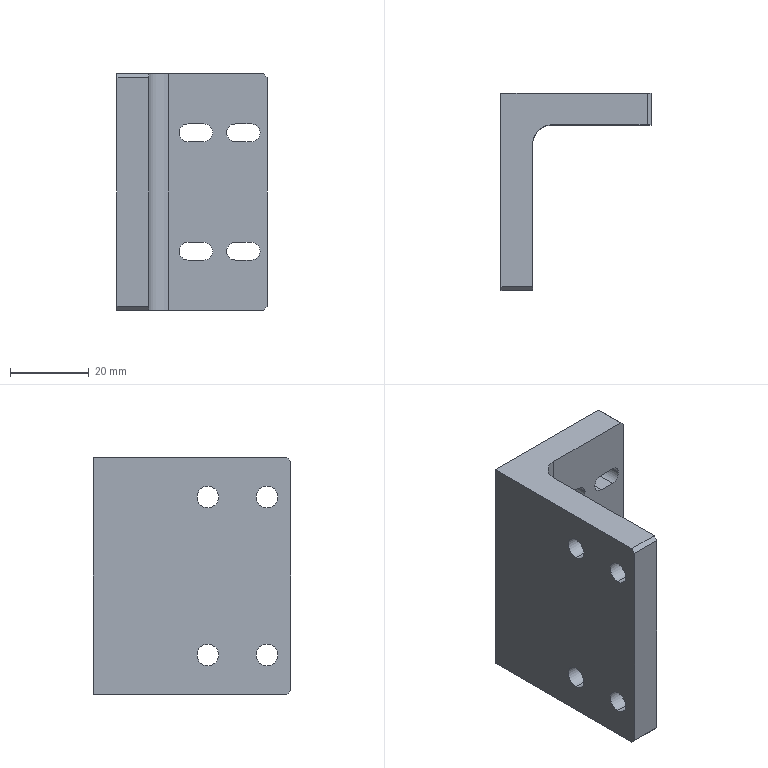Part | NX | features BREP 1 | 1 solid | 41 faces | box 38 x 50 x 60 mm | volume 36861 mm3 | cylinder 21 | plane 20 | commonest cylinder face diameters 4.5 x12 5.5 x8 10 x1
STEP:
#1=CARTESIAN_POINT('',(22.,50.,-12.75));
#2=VERTEX_POINT('',#1);
#3=CARTESIAN_POINT('',(24.25,50.,-15.));
#4=VERTEX_POINT('',#3);
#5=CARTESIAN_POINT('',(22.,50.,-15.));
#6=DIRECTION('',(0.,1.,0.));
#7=DIRECTION('',(0.,0.,1.));
#8=AXIS2_PLACEMENT_3D('',#5,#6,#7);
#9=CIRCLE('',#8,2.25);
#10=EDGE_CURVE('',#2,#4,#9,.T.);
#11=ORIENTED_EDGE('',*,*,#10,.T.);
#12=CARTESIAN_POINT('',(24.25,42.,-15.));
#13=VERTEX_POINT('',#12);
#14=CARTESIAN_POINT('',(24.25,59.,-15.));
#15=DIRECTION('',(0.,-1.,0.));
#16=VECTOR('',#15,1000.);
#17=LINE('',#14,#16);
#18=EDGE_CURVE('',#4,#13,#17,.T.);
#19=ORIENTED_EDGE('',*,*,#18,.T.);
#20=CARTESIAN_POINT('',(22.,42.,-12.75));
#21=VERTEX_POINT('',#20);
#22=CARTESIAN_POINT('',(22.,42.,-15.));
#23=DIRECTION('',(0.,-1.,0.));
#24=DIRECTION('',(1.,0.,0.));
#25=AXIS2_PLACEMENT_3D('',#22,#23,#24);
#26=CIRCLE('',#25,2.25);
#27=EDGE_CURVE('',#13,#21,#26,.T.);
#28=ORIENTED_EDGE('',*,*,#27,.T.);
#29=CARTESIAN_POINT('',(22.,59.,-12.75));
#30=DIRECTION('',(0.,-1.,0.));
#31=VECTOR('',#30,1000.);
#32=LINE('',#29,#31);
#33=EDGE_CURVE('',#2,#21,#32,.T.);
#34=ORIENTED_EDGE('',*,*,#33,.F.);
#35=EDGE_LOOP('',(#11,#19,#28,#34));
#36=FACE_BOUND('',#35,.T.);
#37=CARTESIAN_POINT('',(22.,59.,-15.));
#38=DIRECTION('',(0.,-1.,0.));
#39=DIRECTION('',(1.,0.,0.));
#40=AXIS2_PLACEMENT_3D('',#37,#38,#39);
#41=CYLINDRICAL_SURFACE('',#40,2.25);
#42=ADVANCED_FACE('',(#36),#41,.F.);
#43=CARTESIAN_POINT('',(34.,50.,-12.75));
#44=VERTEX_POINT('',#43);
#45=CARTESIAN_POINT('',(36.25,50.,-15.));
#46=VERTEX_POINT('',#45);
#47=CARTESIAN_POINT('',(34.,50.,-15.));
#48=DIRECTION('',(0.,1.,0.));
#49=DIRECTION('',(0.,0.,1.));
#50=AXIS2_PLACEMENT_3D('',#47,#48,#49);
#51=CIRCLE('',#50,2.25);
#52=EDGE_CURVE('',#44,#46,#51,.T.);
#53=ORIENTED_EDGE('',*,*,#52,.T.);
#54=CARTESIAN_POINT('',(36.25,42.,-15.));
#55=VERTEX_POINT('',#54);
#56=CARTESIAN_POINT('',(36.25,59.,-15.));
#57=DIRECTION('',(0.,-1.,0.));
#58=VECTOR('',#57,1000.);
#59=LINE('',#56,#58);
#60=EDGE_CURVE('',#46,#55,#59,.T.);
#61=ORIENTED_EDGE('',*,*,#60,.T.);
#62=CARTESIAN_POINT('',(34.,42.,-12.75));
#63=VERTEX_POINT('',#62);
#64=CARTESIAN_POINT('',(34.,42.,-15.));
#65=DIRECTION('',(0.,-1.,0.));
#66=DIRECTION('',(1.,0.,0.));
#67=AXIS2_PLACEMENT_3D('',#64,#65,#66);
#68=CIRCLE('',#67,2.25);
#69=EDGE_CURVE('',#55,#63,#68,.T.);
#70=ORIENTED_EDGE('',*,*,#69,.T.);
#71=CARTESIAN_POINT('',(34.,59.,-12.75));
#72=DIRECTION('',(0.,-1.,0.));
#73=VECTOR('',#72,1000.);
#74=LINE('',#71,#73);
#75=EDGE_CURVE('',#44,#63,#74,.T.);
#76=ORIENTED_EDGE('',*,*,#75,.F.);
#77=EDGE_LOOP('',(#53,#61,#70,#76));
#78=FACE_BOUND('',#77,.T.);
#79=CARTESIAN_POINT('',(34.,59.,-15.));
#80=DIRECTION('',(0.,-1.,0.));
#81=DIRECTION('',(1.,0.,0.));
#82=AXIS2_PLACEMENT_3D('',#79,#80,#81);
#83=CYLINDRICAL_SURFACE('',#82,2.25);
#84=ADVANCED_FACE('',(#78),#83,.F.);
#85=CARTESIAN_POINT('',(22.,50.,17.25));
#86=VERTEX_POINT('',#85);
#87=CARTESIAN_POINT('',(24.25,50.,15.));
#88=VERTEX_POINT('',#87);
#89=CARTESIAN_POINT('',(22.,50.,15.));
#90=DIRECTION('',(0.,1.,0.));
#91=DIRECTION('',(0.,0.,1.));
#92=AXIS2_PLACEMENT_3D('',#89,#90,#91);
#93=CIRCLE('',#92,2.25);
#94=EDGE_CURVE('',#86,#88,#93,.T.);
#95=ORIENTED_EDGE('',*,*,#94,.T.);
#96=CARTESIAN_POINT('',(24.25,42.,15.));
#97=VERTEX_POINT('',#96);
#98=CARTESIAN_POINT('',(24.25,59.,15.));
#99=DIRECTION('',(0.,-1.,0.));
#100=VECTOR('',#99,1000.);
#101=LINE('',#98,#100);
#102=EDGE_CURVE('',#88,#97,#101,.T.);
#103=ORIENTED_EDGE('',*,*,#102,.T.);
#104=CARTESIAN_POINT('',(22.,42.,17.25));
#105=VERTEX_POINT('',#104);
#106=CARTESIAN_POINT('',(22.,42.,15.));
#107=DIRECTION('',(0.,-1.,0.));
#108=DIRECTION('',(1.,0.,0.));
#109=AXIS2_PLACEMENT_3D('',#106,#107,#108);
#110=CIRCLE('',#109,2.25);
#111=EDGE_CURVE('',#97,#105,#110,.T.);
#112=ORIENTED_EDGE('',*,*,#111,.T.);
#113=CARTESIAN_POINT('',(22.,59.,17.25));
#114=DIRECTION('',(0.,-1.,0.));
#115=VECTOR('',#114,1000.);
#116=LINE('',#113,#115);
#117=EDGE_CURVE('',#86,#105,#116,.T.);
#118=ORIENTED_EDGE('',*,*,#117,.F.);
#119=EDGE_LOOP('',(#95,#103,#112,#118));
#120=FACE_BOUND('',#119,.T.);
#121=CARTESIAN_POINT('',(22.,59.,15.));
#122=DIRECTION('',(0.,-1.,0.));
#123=DIRECTION('',(1.,0.,0.));
#124=AXIS2_PLACEMENT_3D('',#121,#122,#123);
#125=CYLINDRICAL_SURFACE('',#124,2.25);
#126=ADVANCED_FACE('',(#120),#125,.F.);
#127=CARTESIAN_POINT('',(34.,50.,17.25));
#128=VERTEX_POINT('',#127);
#129=CARTESIAN_POINT('',(36.25,50.,15.));
#130=VERTEX_POINT('',#129);
#131=CARTESIAN_POINT('',(34.,50.,15.));
#132=DIRECTION('',(0.,1.,0.));
#133=DIRECTION('',(0.,0.,1.));
#134=AXIS2_PLACEMENT_3D('',#131,#132,#133);
#135=CIRCLE('',#134,2.25);
#136=EDGE_CURVE('',#128,#130,#135,.T.);
#137=ORIENTED_EDGE('',*,*,#136,.T.);
#138=CARTESIAN_POINT('',(36.25,42.,15.));
#139=VERTEX_POINT('',#138);
#140=CARTESIAN_POINT('',(36.25,59.,15.));
#141=DIRECTION('',(0.,-1.,0.));
#142=VECTOR('',#141,1000.);
#143=LINE('',#140,#142);
#144=EDGE_CURVE('',#130,#139,#143,.T.);
#145=ORIENTED_EDGE('',*,*,#144,.T.);
#146=CARTESIAN_POINT('',(34.,42.,17.25));
#147=VERTEX_POINT('',#146);
#148=CARTESIAN_POINT('',(34.,42.,15.));
#149=DIRECTION('',(0.,-1.,0.));
#150=DIRECTION('',(1.,0.,0.));
#151=AXIS2_PLACEMENT_3D('',#148,#149,#150);
#152=CIRCLE('',#151,2.25);
#153=EDGE_CURVE('',#139,#147,#152,.T.);
#154=ORIENTED_EDGE('',*,*,#153,.T.);
#155=CARTESIAN_POINT('',(34.,59.,17.25));
#156=DIRECTION('',(0.,-1.,0.));
#157=VECTOR('',#156,1000.);
#158=LINE('',#155,#157);
#159=EDGE_CURVE('',#128,#147,#158,.T.);
#160=ORIENTED_EDGE('',*,*,#159,.F.);
#161=EDGE_LOOP('',(#137,#145,#154,#160));
#162=FACE_BOUND('',#161,.T.);
#163=CARTESIAN_POINT('',(34.,59.,15.));
#164=DIRECTION('',(0.,-1.,0.));
#165=DIRECTION('',(1.,0.,0.));
#166=AXIS2_PLACEMENT_3D('',#163,#164,#165);
#167=CYLINDRICAL_SURFACE('',#166,2.25);
#168=ADVANCED_FACE('',(#162),#167,.F.);
#169=CARTESIAN_POINT('',(0.,21.,17.25));
#170=VERTEX_POINT('',#169);
#171=CARTESIAN_POINT('',(0.,21.,22.75));
#172=VERTEX_POINT('',#171);
#173=CARTESIAN_POINT('',(0.,21.,20.));
#174=DIRECTION('',(-1.,0.,0.));
#175=DIRECTION('',(0.,0.,1.));
#176=AXIS2_PLACEMENT_3D('',#173,#174,#175);
#177=CIRCLE('',#176,2.75);
#178=EDGE_CURVE('',#170,#172,#177,.T.);
#179=ORIENTED_EDGE('',*,*,#178,.T.);
#180=CARTESIAN_POINT('',(8.,21.,22.75));
#181=VERTEX_POINT('',#180);
#182=CARTESIAN_POINT('',(8.,21.,22.75));
#183=DIRECTION('',(1.,0.,0.));
#184=VECTOR('',#183,1000.);
#185=LINE('',#182,#184);
#186=EDGE_CURVE('',#172,#181,#185,.T.);
#187=ORIENTED_EDGE('',*,*,#186,.T.);
#188=CARTESIAN_POINT('',(8.,21.,17.25));
#189=VERTEX_POINT('',#188);
#190=CARTESIAN_POINT('',(8.,21.,20.));
#191=DIRECTION('',(1.,0.,0.));
#192=DIRECTION('',(0.,0.,-1.));
#193=AXIS2_PLACEMENT_3D('',#190,#191,#192);
#194=CIRCLE('',#193,2.75);
#195=EDGE_CURVE('',#181,#189,#194,.T.);
#196=ORIENTED_EDGE('',*,*,#195,.T.);
#197=CARTESIAN_POINT('',(8.,21.,17.25));
#198=DIRECTION('',(1.,0.,0.));
#199=VECTOR('',#198,1000.);
#200=LINE('',#197,#199);
#201=EDGE_CURVE('',#170,#189,#200,.T.);
#202=ORIENTED_EDGE('',*,*,#201,.F.);
#203=EDGE_LOOP('',(#179,#187,#196,#202));
#204=FACE_BOUND('',#203,.T.);
#205=CARTESIAN_POINT('',(8.,21.,20.));
#206=DIRECTION('',(1.,0.,0.));
#207=DIRECTION('',(0.,0.,-1.));
#208=AXIS2_PLACEMENT_3D('',#205,#206,#207);
#209=CYLINDRICAL_SURFACE('',#208,2.75);
#210=ADVANCED_FACE('',(#204),#209,.F.);
#211=CARTESIAN_POINT('',(0.,6.,17.25));
#212=VERTEX_POINT('',#211);
#213=CARTESIAN_POINT('',(0.,6.,22.75));
#214=VERTEX_POINT('',#213);
#215=CARTESIAN_POINT('',(0.,6.,20.));
#216=DIRECTION('',(-1.,0.,0.));
#217=DIRECTION('',(0.,0.,1.));
#218=AXIS2_PLACEMENT_3D('',#215,#216,#217);
#219=CIRCLE('',#218,2.75);
#220=EDGE_CURVE('',#212,#214,#219,.T.);
#221=ORIENTED_EDGE('',*,*,#220,.T.);
#222=CARTESIAN_POINT('',(8.,6.,22.75));
#223=VERTEX_POINT('',#222);
#224=CARTESIAN_POINT('',(8.,6.,22.75));
#225=DIRECTION('',(1.,0.,0.));
#226=VECTOR('',#225,1000.);
#227=LINE('',#224,#226);
#228=EDGE_CURVE('',#214,#223,#227,.T.);
#229=ORIENTED_EDGE('',*,*,#228,.T.);
#230=CARTESIAN_POINT('',(8.,6.,17.25));
#231=VERTEX_POINT('',#230);
#232=CARTESIAN_POINT('',(8.,6.,20.));
#233=DIRECTION('',(1.,0.,0.));
#234=DIRECTION('',(0.,0.,-1.));
#235=AXIS2_PLACEMENT_3D('',#232,#233,#234);
#236=CIRCLE('',#235,2.75);
#237=EDGE_CURVE('',#223,#231,#236,.T.);
#238=ORIENTED_EDGE('',*,*,#237,.T.);
#239=CARTESIAN_POINT('',(8.,6.,17.25));
#240=DIRECTION('',(1.,0.,0.));
#241=VECTOR('',#240,1000.);
#242=LINE('',#239,#241);
#243=EDGE_CURVE('',#212,#231,#242,.T.);
#244=ORIENTED_EDGE('',*,*,#243,.F.);
#245=EDGE_LOOP('',(#221,#229,#238,#244));
#246=FACE_BOUND('',#245,.T.);
#247=CARTESIAN_POINT('',(8.,6.,20.));
#248=DIRECTION('',(1.,0.,0.));
#249=DIRECTION('',(0.,0.,-1.));
#250=AXIS2_PLACEMENT_3D('',#247,#248,#249);
#251=CYLINDRICAL_SURFACE('',#250,2.75);
#252=ADVANCED_FACE('',(#246),#251,.F.);
#253=CARTESIAN_POINT('',(0.,6.,-22.75));
#254=VERTEX_POINT('',#253);
#255=CARTESIAN_POINT('',(0.,6.,-17.25));
#256=VERTEX_POINT('',#255);
#257=CARTESIAN_POINT('',(0.,6.,-20.));
#258=DIRECTION('',(-1.,0.,0.));
#259=DIRECTION('',(0.,0.,1.));
#260=AXIS2_PLACEMENT_3D('',#257,#258,#259);
#261=CIRCLE('',#260,2.75);
#262=EDGE_CURVE('',#254,#256,#261,.T.);
#263=ORIENTED_EDGE('',*,*,#262,.T.);
#264=CARTESIAN_POINT('',(8.,6.,-17.25));
#265=VERTEX_POINT('',#264);
#266=CARTESIAN_POINT('',(8.,6.,-17.25));
#267=DIRECTION('',(1.,0.,0.));
#268=VECTOR('',#267,1000.);
#269=LINE('',#266,#268);
#270=EDGE_CURVE('',#256,#265,#269,.T.);
#271=ORIENTED_EDGE('',*,*,#270,.T.);
#272=CARTESIAN_POINT('',(8.,6.,-22.75));
#273=VERTEX_POINT('',#272);
#274=CARTESIAN_POINT('',(8.,6.,-20.));
#275=DIRECTION('',(1.,0.,0.));
#276=DIRECTION('',(0.,0.,-1.));
#277=AXIS2_PLACEMENT_3D('',#274,#275,#276);
#278=CIRCLE('',#277,2.75);
#279=EDGE_CURVE('',#265,#273,#278,.T.);
#280=ORIENTED_EDGE('',*,*,#279,.T.);
#281=CARTESIAN_POINT('',(8.,6.,-22.75));
#282=DIRECTION('',(1.,0.,0.));
#283=VECTOR('',#282,1000.);
#284=LINE('',#281,#283);
#285=EDGE_CURVE('',#254,#273,#284,.T.);
#286=ORIENTED_EDGE('',*,*,#285,.F.);
#287=EDGE_LOOP('',(#263,#271,#280,#286));
#288=FACE_BOUND('',#287,.T.);
#289=CARTESIAN_POINT('',(8.,6.,-20.));
#290=DIRECTION('',(1.,0.,0.));
#291=DIRECTION('',(0.,0.,-1.));
#292=AXIS2_PLACEMENT_3D('',#289,#290,#291);
#293=CYLINDRICAL_SURFACE('',#292,2.75);
#294=ADVANCED_FACE('',(#288),#293,.F.);
#295=CARTESIAN_POINT('',(0.,21.,-22.75));
#296=VERTEX_POINT('',#295);
#297=CARTESIAN_POINT('',(0.,21.,-17.25));
#298=VERTEX_POINT('',#297);
#299=CARTESIAN_POINT('',(0.,21.,-20.));
#300=DIRECTION('',(-1.,0.,0.));
#301=DIRECTION('',(0.,0.,1.));
#302=AXIS2_PLACEMENT_3D('',#299,#300,#301);
#303=CIRCLE('',#302,2.75);
#304=EDGE_CURVE('',#296,#298,#303,.T.);
#305=ORIENTED_EDGE('',*,*,#304,.T.);
#306=CARTESIAN_POINT('',(8.,21.,-17.25));
#307=VERTEX_POINT('',#306);
#308=CARTESIAN_POINT('',(8.,21.,-17.25));
#309=DIRECTION('',(1.,0.,0.));
#310=VECTOR('',#309,1000.);
#311=LINE('',#308,#310);
#312=EDGE_CURVE('',#298,#307,#311,.T.);
#313=ORIENTED_EDGE('',*,*,#312,.T.);
#314=CARTESIAN_POINT('',(8.,21.,-22.75));
#315=VERTEX_POINT('',#314);
#316=CARTESIAN_POINT('',(8.,21.,-20.));
#317=DIRECTION('',(1.,0.,0.));
#318=DIRECTION('',(0.,0.,-1.));
#319=AXIS2_PLACEMENT_3D('',#316,#317,#318);
#320=CIRCLE('',#319,2.75);
#321=EDGE_CURVE('',#307,#315,#320,.T.);
#322=ORIENTED_EDGE('',*,*,#321,.T.);
#323=CARTESIAN_POINT('',(8.,21.,-22.75));
#324=DIRECTION('',(1.,0.,0.));
#325=VECTOR('',#324,1000.);
#326=LINE('',#323,#325);
#327=EDGE_CURVE('',#296,#315,#326,.T.);
#328=ORIENTED_EDGE('',*,*,#327,.F.);
#329=EDGE_LOOP('',(#305,#313,#322,#328));
#330=FACE_BOUND('',#329,.T.);
#331=CARTESIAN_POINT('',(8.,21.,-20.));
#332=DIRECTION('',(1.,0.,0.));
#333=DIRECTION('',(0.,0.,-1.));
#334=AXIS2_PLACEMENT_3D('',#331,#332,#333);
#335=CYLINDRICAL_SURFACE('',#334,2.75);
#336=ADVANCED_FACE('',(#330),#335,.F.);
#337=CARTESIAN_POINT('',(8.,0.,29.));
#338=VERTEX_POINT('',#337);
#339=CARTESIAN_POINT('',(8.,0.,-29.));
#340=VERTEX_POINT('',#339);
#341=CARTESIAN_POINT('',(8.,0.,30.));
#342=DIRECTION('',(0.,0.,-1.));
#343=VECTOR('',#342,1000.);
#344=LINE('',#341,#343);
#345=EDGE_CURVE('',#338,#340,#344,.T.);
#346=ORIENTED_EDGE('',*,*,#345,.T.);
#347=CARTESIAN_POINT('',(8.,1.,-30.));
#348=VERTEX_POINT('',#347);
#349=CARTESIAN_POINT('',(8.,-29.5,0.5));
#350=DIRECTION('',(0.,0.7071,-0.7071));
#351=VECTOR('',#350,1000.);
#352=LINE('',#349,#351);
#353=EDGE_CURVE('',#340,#348,#352,.T.);
#354=ORIENTED_EDGE('',*,*,#353,.T.);
#355=CARTESIAN_POINT('',(8.,37.,-30.));
#356=VERTEX_POINT('',#355);
#357=CARTESIAN_POINT('',(8.,0.,-30.));
#358=DIRECTION('',(0.,-1.,0.));
#359=VECTOR('',#358,1000.);
#360=LINE('',#357,#359);
#361=EDGE_CURVE('',#356,#348,#360,.T.);
#362=ORIENTED_EDGE('',*,*,#361,.F.);
#363=CARTESIAN_POINT('',(8.,37.,30.));
#364=VERTEX_POINT('',#363);
#365=CARTESIAN_POINT('',(8.,37.,30.));
#366=DIRECTION('',(0.,0.,-1.));
#367=VECTOR('',#366,1000.);
#368=LINE('',#365,#367);
#369=EDGE_CURVE('',#364,#356,#368,.T.);
#370=ORIENTED_EDGE('',*,*,#369,.F.);
#371=CARTESIAN_POINT('',(8.,1.,30.));
#372=VERTEX_POINT('',#371);
#373=CARTESIAN_POINT('',(8.,0.,30.));
#374=DIRECTION('',(0.,-1.,0.));
#375=VECTOR('',#374,1000.);
#376=LINE('',#373,#375);
#377=EDGE_CURVE('',#364,#372,#376,.T.);
#378=ORIENTED_EDGE('',*,*,#377,.T.);
#379=CARTESIAN_POINT('',(8.,0.5,29.5));
#380=DIRECTION('',(0.,-0.7071,-0.7071));
#381=VECTOR('',#380,1000.);
#382=LINE('',#379,#381);
#383=EDGE_CURVE('',#372,#338,#382,.T.);
#384=ORIENTED_EDGE('',*,*,#383,.T.);
#385=EDGE_LOOP('',(#346,#354,#362,#370,#378,#384));
#386=FACE_BOUND('',#385,.T.);
#387=CARTESIAN_POINT('',(8.,21.,20.));
#388=DIRECTION('',(1.,0.,0.));
#389=DIRECTION('',(0.,0.,-1.));
#390=AXIS2_PLACEMENT_3D('',#387,#388,#389);
#391=CIRCLE('',#390,2.75);
#392=EDGE_CURVE('',#189,#181,#391,.T.);
#393=ORIENTED_EDGE('',*,*,#392,.F.);
#394=ORIENTED_EDGE('',*,*,#195,.F.);
#395=EDGE_LOOP('',(#393,#394));
#396=FACE_BOUND('',#395,.T.);
#397=CARTESIAN_POINT('',(8.,6.,20.));
#398=DIRECTION('',(1.,0.,0.));
#399=DIRECTION('',(0.,0.,-1.));
#400=AXIS2_PLACEMENT_3D('',#397,#398,#399);
#401=CIRCLE('',#400,2.75);
#402=EDGE_CURVE('',#231,#223,#401,.T.);
#403=ORIENTED_EDGE('',*,*,#402,.F.);
#404=ORIENTED_EDGE('',*,*,#237,.F.);
#405=EDGE_LOOP('',(#403,#404));
#406=FACE_BOUND('',#405,.T.);
#407=CARTESIAN_POINT('',(8.,6.,-20.));
#408=DIRECTION('',(1.,0.,0.));
#409=DIRECTION('',(0.,0.,-1.));
#410=AXIS2_PLACEMENT_3D('',#407,#408,#409);
#411=CIRCLE('',#410,2.75);
#412=EDGE_CURVE('',#273,#265,#411,.T.);
#413=ORIENTED_EDGE('',*,*,#412,.F.);
#414=ORIENTED_EDGE('',*,*,#279,.F.);
#415=EDGE_LOOP('',(#413,#414));
#416=FACE_BOUND('',#415,.T.);
#417=CARTESIAN_POINT('',(8.,21.,-20.));
#418=DIRECTION('',(1.,0.,0.));
#419=DIRECTION('',(0.,0.,-1.));
#420=AXIS2_PLACEMENT_3D('',#417,#418,#419);
#421=CIRCLE('',#420,2.75);
#422=EDGE_CURVE('',#315,#307,#421,.T.);
#423=ORIENTED_EDGE('',*,*,#422,.F.);
#424=ORIENTED_EDGE('',*,*,#321,.F.);
#425=EDGE_LOOP('',(#423,#424));
#426=FACE_BOUND('',#425,.T.);
#427=CARTESIAN_POINT('',(8.,0.,30.));
#428=DIRECTION('',(1.,0.,0.));
#429=DIRECTION('',(0.,1.,0.));
#430=AXIS2_PLACEMENT_3D('',#427,#428,#429);
#431=PLANE('',#430);
#432=ADVANCED_FACE('',(#386,#396,#406,#416,#426),#431,.T.);
#433=CARTESIAN_POINT('',(13.,42.,-30.));
#434=VERTEX_POINT('',#433);
#435=CARTESIAN_POINT('',(13.,37.,-30.));
#436=DIRECTION('',(0.,0.,-1.));
#437=DIRECTION('',(1.,0.,0.));
#438=AXIS2_PLACEMENT_3D('',#435,#436,#437);
#439=CIRCLE('',#438,5.);
#440=EDGE_CURVE('',#356,#434,#439,.T.);
#441=ORIENTED_EDGE('',*,*,#440,.T.);
#442=CARTESIAN_POINT('',(13.,42.,30.));
#443=VERTEX_POINT('',#442);
#444=CARTESIAN_POINT('',(13.,42.,30.));
#445=DIRECTION('',(0.,0.,-1.));
#446=VECTOR('',#445,1000.);
#447=LINE('',#444,#446);
#448=EDGE_CURVE('',#443,#434,#447,.T.);
#449=ORIENTED_EDGE('',*,*,#448,.F.);
#450=CARTESIAN_POINT('',(13.,37.,30.));
#451=DIRECTION('',(0.,0.,-1.));
#452=DIRECTION('',(1.,0.,0.));
#453=AXIS2_PLACEMENT_3D('',#450,#451,#452);
#454=CIRCLE('',#453,5.);
#455=EDGE_CURVE('',#364,#443,#454,.T.);
#456=ORIENTED_EDGE('',*,*,#455,.F.);
#457=ORIENTED_EDGE('',*,*,#369,.T.);
#458=EDGE_LOOP('',(#441,#449,#456,#457));
#459=FACE_BOUND('',#458,.T.);
#460=CARTESIAN_POINT('',(13.,37.,30.));
#461=DIRECTION('',(0.,0.,-1.));
#462=DIRECTION('',(-1.,0.,0.));
#463=AXIS2_PLACEMENT_3D('',#460,#461,#462);
#464=CYLINDRICAL_SURFACE('',#463,5.);
#465=ADVANCED_FACE('',(#459),#464,.F.);
#466=CARTESIAN_POINT('',(38.,42.,29.));
#467=VERTEX_POINT('',#466);
#468=CARTESIAN_POINT('',(38.,42.,-29.));
#469=VERTEX_POINT('',#468);
#470=CARTESIAN_POINT('',(38.,42.,30.));
#471=DIRECTION('',(0.,0.,-1.));
#472=VECTOR('',#471,1000.);
#473=LINE('',#470,#472);
#474=EDGE_CURVE('',#467,#469,#473,.T.);
#475=ORIENTED_EDGE('',*,*,#474,.F.);
#476=CARTESIAN_POINT('',(37.,42.,30.));
#477=VERTEX_POINT('',#476);
#478=CARTESIAN_POINT('',(18.5,42.,48.5));
#479=DIRECTION('',(-0.7071,0.,0.7071));
#480=VECTOR('',#479,1000.);
#481=LINE('',#478,#480);
#482=EDGE_CURVE('',#467,#477,#481,.T.);
#483=ORIENTED_EDGE('',*,*,#482,.T.);
#484=CARTESIAN_POINT('',(0.,42.,30.));
#485=DIRECTION('',(-1.,0.,0.));
#486=VECTOR('',#485,1000.);
#487=LINE('',#484,#486);
#488=EDGE_CURVE('',#477,#443,#487,.T.);
#489=ORIENTED_EDGE('',*,*,#488,.T.);
#490=ORIENTED_EDGE('',*,*,#448,.T.);
#491=CARTESIAN_POINT('',(37.,42.,-30.));
#492=VERTEX_POINT('',#491);
#493=CARTESIAN_POINT('',(0.,42.,-30.));
#494=DIRECTION('',(-1.,0.,0.));
#495=VECTOR('',#494,1000.);
#496=LINE('',#493,#495);
#497=EDGE_CURVE('',#492,#434,#496,.T.);
#498=ORIENTED_EDGE('',*,*,#497,.F.);
#499=CARTESIAN_POINT('',(48.5,42.,-18.5));
#500=DIRECTION('',(0.7071,0.,0.7071));
#501=VECTOR('',#500,1000.);
#502=LINE('',#499,#501);
#503=EDGE_CURVE('',#492,#469,#502,.T.);
#504=ORIENTED_EDGE('',*,*,#503,.T.);
#505=EDGE_LOOP('',(#475,#483,#489,#490,#498,#504));
#506=FACE_BOUND('',#505,.T.);
#507=CARTESIAN_POINT('',(18.,42.,-12.75));
#508=VERTEX_POINT('',#507);
#509=CARTESIAN_POINT('',(18.,42.,-12.75));
#510=DIRECTION('',(-1.,0.,0.));
#511=VECTOR('',#510,1000.);
#512=LINE('',#509,#511);
#513=EDGE_CURVE('',#21,#508,#512,.T.);
#514=ORIENTED_EDGE('',*,*,#513,.F.);
#515=ORIENTED_EDGE('',*,*,#27,.F.);
#516=CARTESIAN_POINT('',(22.,42.,-17.25));
#517=VERTEX_POINT('',#516);
#518=CARTESIAN_POINT('',(22.,42.,-15.));
#519=DIRECTION('',(0.,-1.,0.));
#520=DIRECTION('',(1.,0.,0.));
#521=AXIS2_PLACEMENT_3D('',#518,#519,#520);
#522=CIRCLE('',#521,2.25);
#523=EDGE_CURVE('',#517,#13,#522,.T.);
#524=ORIENTED_EDGE('',*,*,#523,.F.);
#525=CARTESIAN_POINT('',(18.,42.,-17.25));
#526=VERTEX_POINT('',#525);
#527=CARTESIAN_POINT('',(18.,42.,-17.25));
#528=DIRECTION('',(1.,0.,0.));
#529=VECTOR('',#528,1000.);
#530=LINE('',#527,#529);
#531=EDGE_CURVE('',#526,#517,#530,.T.);
#532=ORIENTED_EDGE('',*,*,#531,.F.);
#533=CARTESIAN_POINT('',(18.,42.,-15.));
#534=DIRECTION('',(0.,-1.,0.));
#535=DIRECTION('',(1.,0.,0.));
#536=AXIS2_PLACEMENT_3D('',#533,#534,#535);
#537=CIRCLE('',#536,2.25);
#538=EDGE_CURVE('',#508,#526,#537,.T.);
#539=ORIENTED_EDGE('',*,*,#538,.F.);
#540=EDGE_LOOP('',(#514,#515,#524,#532,#539));
#541=FACE_BOUND('',#540,.T.);
#542=CARTESIAN_POINT('',(30.,42.,-12.75));
#543=VERTEX_POINT('',#542);
#544=CARTESIAN_POINT('',(30.,42.,-12.75));
#545=DIRECTION('',(-1.,0.,0.));
#546=VECTOR('',#545,1000.);
#547=LINE('',#544,#546);
#548=EDGE_CURVE('',#63,#543,#547,.T.);
#549=ORIENTED_EDGE('',*,*,#548,.F.);
#550=ORIENTED_EDGE('',*,*,#69,.F.);
#551=CARTESIAN_POINT('',(34.,42.,-17.25));
#552=VERTEX_POINT('',#551);
#553=CARTESIAN_POINT('',(34.,42.,-15.));
#554=DIRECTION('',(0.,-1.,0.));
#555=DIRECTION('',(1.,0.,0.));
#556=AXIS2_PLACEMENT_3D('',#553,#554,#555);
#557=CIRCLE('',#556,2.25);
#558=EDGE_CURVE('',#552,#55,#557,.T.);
#559=ORIENTED_EDGE('',*,*,#558,.F.);
#560=CARTESIAN_POINT('',(30.,42.,-17.25));
#561=VERTEX_POINT('',#560);
#562=CARTESIAN_POINT('',(30.,42.,-17.25));
#563=DIRECTION('',(1.,0.,0.));
#564=VECTOR('',#563,1000.);
#565=LINE('',#562,#564);
#566=EDGE_CURVE('',#561,#552,#565,.T.);
#567=ORIENTED_EDGE('',*,*,#566,.F.);
#568=CARTESIAN_POINT('',(30.,42.,-15.));
#569=DIRECTION('',(0.,-1.,0.));
#570=DIRECTION('',(1.,0.,0.));
#571=AXIS2_PLACEMENT_3D('',#568,#569,#570);
#572=CIRCLE('',#571,2.25);
#573=EDGE_CURVE('',#543,#561,#572,.T.);
#574=ORIENTED_EDGE('',*,*,#573,.F.);
#575=EDGE_LOOP('',(#549,#550,#559,#567,#574));
#576=FACE_BOUND('',#575,.T.);
#577=CARTESIAN_POINT('',(18.,42.,17.25));
#578=VERTEX_POINT('',#577);
#579=CARTESIAN_POINT('',(18.,42.,17.25));
#580=DIRECTION('',(-1.,0.,0.));
#581=VECTOR('',#580,1000.);
#582=LINE('',#579,#581);
#583=EDGE_CURVE('',#105,#578,#582,.T.);
#584=ORIENTED_EDGE('',*,*,#583,.F.);
#585=ORIENTED_EDGE('',*,*,#111,.F.);
#586=CARTESIAN_POINT('',(22.,42.,12.75));
#587=VERTEX_POINT('',#586);
#588=CARTESIAN_POINT('',(22.,42.,15.));
#589=DIRECTION('',(0.,-1.,0.));
#590=DIRECTION('',(1.,0.,0.));
#591=AXIS2_PLACEMENT_3D('',#588,#589,#590);
#592=CIRCLE('',#591,2.25);
#593=EDGE_CURVE('',#587,#97,#592,.T.);
#594=ORIENTED_EDGE('',*,*,#593,.F.);
#595=CARTESIAN_POINT('',(18.,42.,12.75));
#596=VERTEX_POINT('',#595);
#597=CARTESIAN_POINT('',(18.,42.,12.75));
#598=DIRECTION('',(1.,0.,0.));
#599=VECTOR('',#598,1000.);
#600=LINE('',#597,#599);
#601=EDGE_CURVE('',#596,#587,#600,.T.);
#602=ORIENTED_EDGE('',*,*,#601,.F.);
#603=CARTESIAN_POINT('',(18.,42.,15.));
#604=DIRECTION('',(0.,-1.,0.));
#605=DIRECTION('',(1.,0.,0.));
#606=AXIS2_PLACEMENT_3D('',#603,#604,#605);
#607=CIRCLE('',#606,2.25);
#608=EDGE_CURVE('',#578,#596,#607,.T.);
#609=ORIENTED_EDGE('',*,*,#608,.F.);
#610=EDGE_LOOP('',(#584,#585,#594,#602,#609));
#611=FACE_BOUND('',#610,.T.);
#612=CARTESIAN_POINT('',(30.,42.,17.25));
#613=VERTEX_POINT('',#612);
#614=CARTESIAN_POINT('',(30.,42.,17.25));
#615=DIRECTION('',(-1.,0.,0.));
#616=VECTOR('',#615,1000.);
#617=LINE('',#614,#616);
#618=EDGE_CURVE('',#147,#613,#617,.T.);
#619=ORIENTED_EDGE('',*,*,#618,.F.);
#620=ORIENTED_EDGE('',*,*,#153,.F.);
#621=CARTESIAN_POINT('',(34.,42.,12.75));
#622=VERTEX_POINT('',#621);
#623=CARTESIAN_POINT('',(34.,42.,15.));
#624=DIRECTION('',(0.,-1.,0.));
#625=DIRECTION('',(1.,0.,0.));
#626=AXIS2_PLACEMENT_3D('',#623,#624,#625);
#627=CIRCLE('',#626,2.25);
#628=EDGE_CURVE('',#622,#139,#627,.T.);
#629=ORIENTED_EDGE('',*,*,#628,.F.);
#630=CARTESIAN_POINT('',(30.,42.,12.75));
#631=VERTEX_POINT('',#630);
#632=CARTESIAN_POINT('',(30.,42.,12.75));
#633=DIRECTION('',(1.,0.,0.));
#634=VECTOR('',#633,1000.);
#635=LINE('',#632,#634);
#636=EDGE_CURVE('',#631,#622,#635,.T.);
#637=ORIENTED_EDGE('',*,*,#636,.F.);
#638=CARTESIAN_POINT('',(30.,42.,15.));
#639=DIRECTION('',(0.,-1.,0.));
#640=DIRECTION('',(1.,0.,0.));
#641=AXIS2_PLACEMENT_3D('',#638,#639,#640);
#642=CIRCLE('',#641,2.25);
#643=EDGE_CURVE('',#613,#631,#642,.T.);
#644=ORIENTED_EDGE('',*,*,#643,.F.);
#645=EDGE_LOOP('',(#619,#620,#629,#637,#644));
#646=FACE_BOUND('',#645,.T.);
#647=CARTESIAN_POINT('',(0.,42.,30.));
#648=DIRECTION('',(0.,-1.,0.));
#649=DIRECTION('',(0.,0.,-1.));
#650=AXIS2_PLACEMENT_3D('',#647,#648,#649);
#651=PLANE('',#650);
#652=ADVANCED_FACE('',(#506,#541,#576,#611,#646),#651,.T.);
#653=CARTESIAN_POINT('',(38.,50.,29.));
#654=VERTEX_POINT('',#653);
#655=CARTESIAN_POINT('',(38.,50.,-29.));
#656=VERTEX_POINT('',#655);
#657=CARTESIAN_POINT('',(38.,50.,30.));
#658=DIRECTION('',(0.,0.,-1.));
#659=VECTOR('',#658,1000.);
#660=LINE('',#657,#659);
#661=EDGE_CURVE('',#654,#656,#660,.T.);
#662=ORIENTED_EDGE('',*,*,#661,.F.);
#663=CARTESIAN_POINT('',(38.,0.,29.));
#664=DIRECTION('',(0.,-1.,0.));
#665=VECTOR('',#664,1000.);
#666=LINE('',#663,#665);
#667=EDGE_CURVE('',#654,#467,#666,.T.);
#668=ORIENTED_EDGE('',*,*,#667,.T.);
#669=ORIENTED_EDGE('',*,*,#474,.T.);
#670=CARTESIAN_POINT('',(38.,50.,-29.));
#671=DIRECTION('',(0.,1.,0.));
#672=VECTOR('',#671,1000.);
#673=LINE('',#670,#672);
#674=EDGE_CURVE('',#469,#656,#673,.T.);
#675=ORIENTED_EDGE('',*,*,#674,.T.);
#676=EDGE_LOOP('',(#662,#668,#669,#675));
#677=FACE_BOUND('',#676,.T.);
#678=CARTESIAN_POINT('',(38.,0.,30.));
#679=DIRECTION('',(1.,0.,0.));
#680=DIRECTION('',(0.,1.,0.));
#681=AXIS2_PLACEMENT_3D('',#678,#679,#680);
#682=PLANE('',#681);
#683=ADVANCED_FACE('',(#677),#682,.T.);
#684=CARTESIAN_POINT('',(0.,50.,30.));
#685=VERTEX_POINT('',#684);
#686=CARTESIAN_POINT('',(37.,50.,30.));
#687=VERTEX_POINT('',#686);
#688=CARTESIAN_POINT('',(0.,50.,30.));
#689=DIRECTION('',(1.,0.,0.));
#690=VECTOR('',#689,1000.);
#691=LINE('',#688,#690);
#692=EDGE_CURVE('',#685,#687,#691,.T.);
#693=ORIENTED_EDGE('',*,*,#692,.T.);
#694=CARTESIAN_POINT('',(18.5,50.,48.5));
#695=DIRECTION('',(0.7071,0.,-0.7071));
#696=VECTOR('',#695,1000.);
#697=LINE('',#694,#696);
#698=EDGE_CURVE('',#687,#654,#697,.T.);
#699=ORIENTED_EDGE('',*,*,#698,.T.);
#700=ORIENTED_EDGE('',*,*,#661,.T.);
#701=CARTESIAN_POINT('',(37.,50.,-30.));
#702=VERTEX_POINT('',#701);
#703=CARTESIAN_POINT('',(48.5,50.,-18.5));
#704=DIRECTION('',(-0.7071,0.,-0.7071));
#705=VECTOR('',#704,1000.);
#706=LINE('',#703,#705);
#707=EDGE_CURVE('',#656,#702,#706,.T.);
#708=ORIENTED_EDGE('',*,*,#707,.T.);
#709=CARTESIAN_POINT('',(0.,50.,-30.));
#710=VERTEX_POINT('',#709);
#711=CARTESIAN_POINT('',(0.,50.,-30.));
#712=DIRECTION('',(1.,0.,0.));
#713=VECTOR('',#712,1000.);
#714=LINE('',#711,#713);
#715=EDGE_CURVE('',#710,#702,#714,.T.);
#716=ORIENTED_EDGE('',*,*,#715,.F.);
#717=CARTESIAN_POINT('',(0.,50.,30.));
#718=DIRECTION('',(0.,0.,-1.));
#719=VECTOR('',#718,1000.);
#720=LINE('',#717,#719);
#721=EDGE_CURVE('',#685,#710,#720,.T.);
#722=ORIENTED_EDGE('',*,*,#721,.F.);
#723=EDGE_LOOP('',(#693,#699,#700,#708,#716,#722));
#724=FACE_BOUND('',#723,.T.);
#725=CARTESIAN_POINT('',(18.,50.,-17.25));
#726=VERTEX_POINT('',#725);
#727=CARTESIAN_POINT('',(18.,50.,-12.75));
#728=VERTEX_POINT('',#727);
#729=CARTESIAN_POINT('',(18.,50.,-15.));
#730=DIRECTION('',(0.,1.,0.));
#731=DIRECTION('',(0.,0.,1.));
#732=AXIS2_PLACEMENT_3D('',#729,#730,#731);
#733=CIRCLE('',#732,2.25);
#734=EDGE_CURVE('',#726,#728,#733,.T.);
#735=ORIENTED_EDGE('',*,*,#734,.F.);
#736=CARTESIAN_POINT('',(22.,50.,-17.25));
#737=VERTEX_POINT('',#736);
#738=CARTESIAN_POINT('',(0.,50.,-17.25));
#739=DIRECTION('',(-1.,0.,0.));
#740=VECTOR('',#739,1000.);
#741=LINE('',#738,#740);
#742=EDGE_CURVE('',#737,#726,#741,.T.);
#743=ORIENTED_EDGE('',*,*,#742,.F.);
#744=CARTESIAN_POINT('',(22.,50.,-15.));
#745=DIRECTION('',(0.,1.,0.));
#746=DIRECTION('',(0.,0.,1.));
#747=AXIS2_PLACEMENT_3D('',#744,#745,#746);
#748=CIRCLE('',#747,2.25);
#749=EDGE_CURVE('',#4,#737,#748,.T.);
#750=ORIENTED_EDGE('',*,*,#749,.F.);
#751=ORIENTED_EDGE('',*,*,#10,.F.);
#752=CARTESIAN_POINT('',(0.,50.,-12.75));
#753=DIRECTION('',(1.,0.,0.));
#754=VECTOR('',#753,1000.);
#755=LINE('',#752,#754);
#756=EDGE_CURVE('',#728,#2,#755,.T.);
#757=ORIENTED_EDGE('',*,*,#756,.F.);
#758=EDGE_LOOP('',(#735,#743,#750,#751,#757));
#759=FACE_BOUND('',#758,.T.);
#760=CARTESIAN_POINT('',(30.,50.,-17.25));
#761=VERTEX_POINT('',#760);
#762=CARTESIAN_POINT('',(30.,50.,-12.75));
#763=VERTEX_POINT('',#762);
#764=CARTESIAN_POINT('',(30.,50.,-15.));
#765=DIRECTION('',(0.,1.,0.));
#766=DIRECTION('',(0.,0.,1.));
#767=AXIS2_PLACEMENT_3D('',#764,#765,#766);
#768=CIRCLE('',#767,2.25);
#769=EDGE_CURVE('',#761,#763,#768,.T.);
#770=ORIENTED_EDGE('',*,*,#769,.F.);
#771=CARTESIAN_POINT('',(34.,50.,-17.25));
#772=VERTEX_POINT('',#771);
#773=CARTESIAN_POINT('',(0.,50.,-17.25));
#774=DIRECTION('',(-1.,0.,0.));
#775=VECTOR('',#774,1000.);
#776=LINE('',#773,#775);
#777=EDGE_CURVE('',#772,#761,#776,.T.);
#778=ORIENTED_EDGE('',*,*,#777,.F.);
#779=CARTESIAN_POINT('',(34.,50.,-15.));
#780=DIRECTION('',(0.,1.,0.));
#781=DIRECTION('',(0.,0.,1.));
#782=AXIS2_PLACEMENT_3D('',#779,#780,#781);
#783=CIRCLE('',#782,2.25);
#784=EDGE_CURVE('',#46,#772,#783,.T.);
#785=ORIENTED_EDGE('',*,*,#784,.F.);
#786=ORIENTED_EDGE('',*,*,#52,.F.);
#787=CARTESIAN_POINT('',(0.,50.,-12.75));
#788=DIRECTION('',(1.,0.,0.));
#789=VECTOR('',#788,1000.);
#790=LINE('',#787,#789);
#791=EDGE_CURVE('',#763,#44,#790,.T.);
#792=ORIENTED_EDGE('',*,*,#791,.F.);
#793=EDGE_LOOP('',(#770,#778,#785,#786,#792));
#794=FACE_BOUND('',#793,.T.);
#795=CARTESIAN_POINT('',(18.,50.,12.75));
#796=VERTEX_POINT('',#795);
#797=CARTESIAN_POINT('',(18.,50.,17.25));
#798=VERTEX_POINT('',#797);
#799=CARTESIAN_POINT('',(18.,50.,15.));
#800=DIRECTION('',(0.,1.,0.));
#801=DIRECTION('',(0.,0.,1.));
#802=AXIS2_PLACEMENT_3D('',#799,#800,#801);
#803=CIRCLE('',#802,2.25);
#804=EDGE_CURVE('',#796,#798,#803,.T.);
#805=ORIENTED_EDGE('',*,*,#804,.F.);
#806=CARTESIAN_POINT('',(22.,50.,12.75));
#807=VERTEX_POINT('',#806);
#808=CARTESIAN_POINT('',(0.,50.,12.75));
#809=DIRECTION('',(-1.,0.,0.));
#810=VECTOR('',#809,1000.);
#811=LINE('',#808,#810);
#812=EDGE_CURVE('',#807,#796,#811,.T.);
#813=ORIENTED_EDGE('',*,*,#812,.F.);
#814=CARTESIAN_POINT('',(22.,50.,15.));
#815=DIRECTION('',(0.,1.,0.));
#816=DIRECTION('',(0.,0.,1.));
#817=AXIS2_PLACEMENT_3D('',#814,#815,#816);
#818=CIRCLE('',#817,2.25);
#819=EDGE_CURVE('',#88,#807,#818,.T.);
#820=ORIENTED_EDGE('',*,*,#819,.F.);
#821=ORIENTED_EDGE('',*,*,#94,.F.);
#822=CARTESIAN_POINT('',(0.,50.,17.25));
#823=DIRECTION('',(1.,0.,0.));
#824=VECTOR('',#823,1000.);
#825=LINE('',#822,#824);
#826=EDGE_CURVE('',#798,#86,#825,.T.);
#827=ORIENTED_EDGE('',*,*,#826,.F.);
#828=EDGE_LOOP('',(#805,#813,#820,#821,#827));
#829=FACE_BOUND('',#828,.T.);
#830=CARTESIAN_POINT('',(30.,50.,12.75));
#831=VERTEX_POINT('',#830);
#832=CARTESIAN_POINT('',(30.,50.,17.25));
#833=VERTEX_POINT('',#832);
#834=CARTESIAN_POINT('',(30.,50.,15.));
#835=DIRECTION('',(0.,1.,0.));
#836=DIRECTION('',(0.,0.,1.));
#837=AXIS2_PLACEMENT_3D('',#834,#835,#836);
#838=CIRCLE('',#837,2.25);
#839=EDGE_CURVE('',#831,#833,#838,.T.);
#840=ORIENTED_EDGE('',*,*,#839,.F.);
#841=CARTESIAN_POINT('',(34.,50.,12.75));
#842=VERTEX_POINT('',#841);
#843=CARTESIAN_POINT('',(0.,50.,12.75));
#844=DIRECTION('',(-1.,0.,0.));
#845=VECTOR('',#844,1000.);
#846=LINE('',#843,#845);
#847=EDGE_CURVE('',#842,#831,#846,.T.);
#848=ORIENTED_EDGE('',*,*,#847,.F.);
#849=CARTESIAN_POINT('',(34.,50.,15.));
#850=DIRECTION('',(0.,1.,0.));
#851=DIRECTION('',(0.,0.,1.));
#852=AXIS2_PLACEMENT_3D('',#849,#850,#851);
#853=CIRCLE('',#852,2.25);
#854=EDGE_CURVE('',#130,#842,#853,.T.);
#855=ORIENTED_EDGE('',*,*,#854,.F.);
#856=ORIENTED_EDGE('',*,*,#136,.F.);
#857=CARTESIAN_POINT('',(0.,50.,17.25));
#858=DIRECTION('',(1.,0.,0.));
#859=VECTOR('',#858,1000.);
#860=LINE('',#857,#859);
#861=EDGE_CURVE('',#833,#128,#860,.T.);
#862=ORIENTED_EDGE('',*,*,#861,.F.);
#863=EDGE_LOOP('',(#840,#848,#855,#856,#862));
#864=FACE_BOUND('',#863,.T.);
#865=CARTESIAN_POINT('',(0.,50.,30.));
#866=DIRECTION('',(0.,1.,0.));
#867=DIRECTION('',(1.,0.,0.));
#868=AXIS2_PLACEMENT_3D('',#865,#866,#867);
#869=PLANE('',#868);
#870=ADVANCED_FACE('',(#724,#759,#794,#829,#864),#869,.T.);
#871=CARTESIAN_POINT('',(0.,1.,-30.));
#872=VERTEX_POINT('',#871);
#873=CARTESIAN_POINT('',(0.,0.,-30.));
#874=DIRECTION('',(0.,1.,0.));
#875=VECTOR('',#874,1000.);
#876=LINE('',#873,#875);
#877=EDGE_CURVE('',#872,#710,#876,.T.);
#878=ORIENTED_EDGE('',*,*,#877,.F.);
#879=CARTESIAN_POINT('',(0.,0.,-29.));
#880=VERTEX_POINT('',#879);
#881=CARTESIAN_POINT('',(0.,-29.5,0.5));
#882=DIRECTION('',(0.,-0.7071,0.7071));
#883=VECTOR('',#882,1000.);
#884=LINE('',#881,#883);
#885=EDGE_CURVE('',#872,#880,#884,.T.);
#886=ORIENTED_EDGE('',*,*,#885,.T.);
#887=CARTESIAN_POINT('',(0.,0.,29.));
#888=VERTEX_POINT('',#887);
#889=CARTESIAN_POINT('',(0.,0.,30.));
#890=DIRECTION('',(0.,0.,-1.));
#891=VECTOR('',#890,1000.);
#892=LINE('',#889,#891);
#893=EDGE_CURVE('',#888,#880,#892,.T.);
#894=ORIENTED_EDGE('',*,*,#893,.F.);
#895=CARTESIAN_POINT('',(0.,1.,30.));
#896=VERTEX_POINT('',#895);
#897=CARTESIAN_POINT('',(0.,0.5,29.5));
#898=DIRECTION('',(0.,0.7071,0.7071));
#899=VECTOR('',#898,1000.);
#900=LINE('',#897,#899);
#901=EDGE_CURVE('',#888,#896,#900,.T.);
#902=ORIENTED_EDGE('',*,*,#901,.T.);
#903=CARTESIAN_POINT('',(0.,0.,30.));
#904=DIRECTION('',(0.,1.,0.));
#905=VECTOR('',#904,1000.);
#906=LINE('',#903,#905);
#907=EDGE_CURVE('',#896,#685,#906,.T.);
#908=ORIENTED_EDGE('',*,*,#907,.T.);
#909=ORIENTED_EDGE('',*,*,#721,.T.);
#910=EDGE_LOOP('',(#878,#886,#894,#902,#908,#909));
#911=FACE_BOUND('',#910,.T.);
#912=ORIENTED_EDGE('',*,*,#178,.F.);
#913=CARTESIAN_POINT('',(0.,21.,20.));
#914=DIRECTION('',(-1.,0.,0.));
#915=DIRECTION('',(0.,0.,1.));
#916=AXIS2_PLACEMENT_3D('',#913,#914,#915);
#917=CIRCLE('',#916,2.75);
#918=EDGE_CURVE('',#172,#170,#917,.T.);
#919=ORIENTED_EDGE('',*,*,#918,.F.);
#920=EDGE_LOOP('',(#912,#919));
#921=FACE_BOUND('',#920,.T.);
#922=ORIENTED_EDGE('',*,*,#220,.F.);
#923=CARTESIAN_POINT('',(0.,6.,20.));
#924=DIRECTION('',(-1.,0.,0.));
#925=DIRECTION('',(0.,0.,1.));
#926=AXIS2_PLACEMENT_3D('',#923,#924,#925);
#927=CIRCLE('',#926,2.75);
#928=EDGE_CURVE('',#214,#212,#927,.T.);
#929=ORIENTED_EDGE('',*,*,#928,.F.);
#930=EDGE_LOOP('',(#922,#929));
#931=FACE_BOUND('',#930,.T.);
#932=ORIENTED_EDGE('',*,*,#262,.F.);
#933=CARTESIAN_POINT('',(0.,6.,-20.));
#934=DIRECTION('',(-1.,0.,0.));
#935=DIRECTION('',(0.,0.,1.));
#936=AXIS2_PLACEMENT_3D('',#933,#934,#935);
#937=CIRCLE('',#936,2.75);
#938=EDGE_CURVE('',#256,#254,#937,.T.);
#939=ORIENTED_EDGE('',*,*,#938,.F.);
#940=EDGE_LOOP('',(#932,#939));
#941=FACE_BOUND('',#940,.T.);
#942=ORIENTED_EDGE('',*,*,#304,.F.);
#943=CARTESIAN_POINT('',(0.,21.,-20.));
#944=DIRECTION('',(-1.,0.,0.));
#945=DIRECTION('',(0.,0.,1.));
#946=AXIS2_PLACEMENT_3D('',#943,#944,#945);
#947=CIRCLE('',#946,2.75);
#948=EDGE_CURVE('',#298,#296,#947,.T.);
#949=ORIENTED_EDGE('',*,*,#948,.F.);
#950=EDGE_LOOP('',(#942,#949));
#951=FACE_BOUND('',#950,.T.);
#952=CARTESIAN_POINT('',(0.,0.,30.));
#953=DIRECTION('',(-1.,0.,0.));
#954=DIRECTION('',(0.,0.,1.));
#955=AXIS2_PLACEMENT_3D('',#952,#953,#954);
#956=PLANE('',#955);
#957=ADVANCED_FACE('',(#911,#921,#931,#941,#951),#956,.T.);
#958=ORIENTED_EDGE('',*,*,#893,.T.);
#959=CARTESIAN_POINT('',(8.,0.,-29.));
#960=DIRECTION('',(1.,0.,0.));
#961=VECTOR('',#960,1000.);
#962=LINE('',#959,#961);
#963=EDGE_CURVE('',#880,#340,#962,.T.);
#964=ORIENTED_EDGE('',*,*,#963,.T.);
#965=ORIENTED_EDGE('',*,*,#345,.F.);
#966=CARTESIAN_POINT('',(0.,0.,29.));
#967=DIRECTION('',(-1.,0.,0.));
#968=VECTOR('',#967,1000.);
#969=LINE('',#966,#968);
#970=EDGE_CURVE('',#338,#888,#969,.T.);
#971=ORIENTED_EDGE('',*,*,#970,.T.);
#972=EDGE_LOOP('',(#958,#964,#965,#971));
#973=FACE_BOUND('',#972,.T.);
#974=CARTESIAN_POINT('',(0.,0.,30.));
#975=DIRECTION('',(0.,-1.,0.));
#976=DIRECTION('',(-1.,0.,0.));
#977=AXIS2_PLACEMENT_3D('',#974,#975,#976);
#978=PLANE('',#977);
#979=ADVANCED_FACE('',(#973),#978,.T.);
#980=ORIENTED_EDGE('',*,*,#907,.F.);
#981=CARTESIAN_POINT('',(0.,1.,30.));
#982=DIRECTION('',(1.,0.,0.));
#983=VECTOR('',#982,1000.);
#984=LINE('',#981,#983);
#985=EDGE_CURVE('',#896,#372,#984,.T.);
#986=ORIENTED_EDGE('',*,*,#985,.T.);
#987=ORIENTED_EDGE('',*,*,#377,.F.);
#988=ORIENTED_EDGE('',*,*,#455,.T.);
#989=ORIENTED_EDGE('',*,*,#488,.F.);
#990=CARTESIAN_POINT('',(37.,0.,30.));
#991=DIRECTION('',(0.,1.,0.));
#992=VECTOR('',#991,1000.);
#993=LINE('',#990,#992);
#994=EDGE_CURVE('',#477,#687,#993,.T.);
#995=ORIENTED_EDGE('',*,*,#994,.T.);
#996=ORIENTED_EDGE('',*,*,#692,.F.);
#997=EDGE_LOOP('',(#980,#986,#987,#988,#989,#995,#996));
#998=FACE_BOUND('',#997,.T.);
#999=CARTESIAN_POINT('',(0.,0.,30.));
#1000=DIRECTION('',(0.,0.,1.));
#1001=DIRECTION('',(1.,0.,0.));
#1002=AXIS2_PLACEMENT_3D('',#999,#1000,#1001);
#1003=PLANE('',#1002);
#1004=ADVANCED_FACE('',(#998),#1003,.T.);
#1005=ORIENTED_EDGE('',*,*,#361,.T.);
#1006=CARTESIAN_POINT('',(0.,1.,-30.));
#1007=DIRECTION('',(-1.,0.,0.));
#1008=VECTOR('',#1007,1000.);
#1009=LINE('',#1006,#1008);
#1010=EDGE_CURVE('',#348,#872,#1009,.T.);
#1011=ORIENTED_EDGE('',*,*,#1010,.T.);
#1012=ORIENTED_EDGE('',*,*,#877,.T.);
#1013=ORIENTED_EDGE('',*,*,#715,.T.);
#1014=CARTESIAN_POINT('',(37.,42.,-30.));
#1015=DIRECTION('',(0.,-1.,0.));
#1016=VECTOR('',#1015,1000.);
#1017=LINE('',#1014,#1016);
#1018=EDGE_CURVE('',#702,#492,#1017,.T.);
#1019=ORIENTED_EDGE('',*,*,#1018,.T.);
#1020=ORIENTED_EDGE('',*,*,#497,.T.);
#1021=ORIENTED_EDGE('',*,*,#440,.F.);
#1022=EDGE_LOOP('',(#1005,#1011,#1012,#1013,#1019,#1020,#1021));
#1023=FACE_BOUND('',#1022,.T.);
#1024=CARTESIAN_POINT('',(0.,0.,-30.));
#1025=DIRECTION('',(0.,0.,1.));
#1026=DIRECTION('',(1.,0.,0.));
#1027=AXIS2_PLACEMENT_3D('',#1024,#1025,#1026);
#1028=PLANE('',#1027);
#1029=ADVANCED_FACE('',(#1023),#1028,.F.);
#1030=ORIENTED_EDGE('',*,*,#353,.F.);
#1031=ORIENTED_EDGE('',*,*,#963,.F.);
#1032=ORIENTED_EDGE('',*,*,#885,.F.);
#1033=ORIENTED_EDGE('',*,*,#1010,.F.);
#1034=EDGE_LOOP('',(#1030,#1031,#1032,#1033));
#1035=FACE_BOUND('',#1034,.T.);
#1036=CARTESIAN_POINT('',(0.,1.,-30.));
#1037=DIRECTION('',(0.,-0.7071,-0.7071));
#1038=DIRECTION('',(0.,0.7071,-0.7071));
#1039=AXIS2_PLACEMENT_3D('',#1036,#1037,#1038);
#1040=PLANE('',#1039);
#1041=ADVANCED_FACE('',(#1035),#1040,.T.);
#1042=ORIENTED_EDGE('',*,*,#383,.F.);
#1043=ORIENTED_EDGE('',*,*,#985,.F.);
#1044=ORIENTED_EDGE('',*,*,#901,.F.);
#1045=ORIENTED_EDGE('',*,*,#970,.F.);
#1046=EDGE_LOOP('',(#1042,#1043,#1044,#1045));
#1047=FACE_BOUND('',#1046,.T.);
#1048=CARTESIAN_POINT('',(0.,0.,29.));
#1049=DIRECTION('',(0.,0.7071,-0.7071));
#1050=DIRECTION('',(-1.,0.,0.));
#1051=AXIS2_PLACEMENT_3D('',#1048,#1049,#1050);
#1052=PLANE('',#1051);
#1053=ADVANCED_FACE('',(#1047),#1052,.F.);
#1054=ORIENTED_EDGE('',*,*,#698,.F.);
#1055=ORIENTED_EDGE('',*,*,#994,.F.);
#1056=ORIENTED_EDGE('',*,*,#482,.F.);
#1057=ORIENTED_EDGE('',*,*,#667,.F.);
#1058=EDGE_LOOP('',(#1054,#1055,#1056,#1057));
#1059=FACE_BOUND('',#1058,.T.);
#1060=CARTESIAN_POINT('',(38.,0.,29.));
#1061=DIRECTION('',(-0.7071,0.,-0.7071));
#1062=DIRECTION('',(-0.7071,0.,0.7071));
#1063=AXIS2_PLACEMENT_3D('',#1060,#1061,#1062);
#1064=PLANE('',#1063);
#1065=ADVANCED_FACE('',(#1059),#1064,.F.);
#1066=ORIENTED_EDGE('',*,*,#707,.F.);
#1067=ORIENTED_EDGE('',*,*,#674,.F.);
#1068=ORIENTED_EDGE('',*,*,#503,.F.);
#1069=ORIENTED_EDGE('',*,*,#1018,.F.);
#1070=EDGE_LOOP('',(#1066,#1067,#1068,#1069));
#1071=FACE_BOUND('',#1070,.T.);
#1072=CARTESIAN_POINT('',(37.,0.,-30.));
#1073=DIRECTION('',(0.7071,0.,-0.7071));
#1074=DIRECTION('',(0.,-1.,0.));
#1075=AXIS2_PLACEMENT_3D('',#1072,#1073,#1074);
#1076=PLANE('',#1075);
#1077=ADVANCED_FACE('',(#1071),#1076,.T.);
#1078=ORIENTED_EDGE('',*,*,#312,.F.);
#1079=ORIENTED_EDGE('',*,*,#948,.T.);
#1080=ORIENTED_EDGE('',*,*,#327,.T.);
#1081=ORIENTED_EDGE('',*,*,#422,.T.);
#1082=EDGE_LOOP('',(#1078,#1079,#1080,#1081));
#1083=FACE_BOUND('',#1082,.T.);
#1084=CARTESIAN_POINT('',(8.,21.,-20.));
#1085=DIRECTION('',(1.,0.,0.));
#1086=DIRECTION('',(0.,0.,-1.));
#1087=AXIS2_PLACEMENT_3D('',#1084,#1085,#1086);
#1088=CYLINDRICAL_SURFACE('',#1087,2.75);
#1089=ADVANCED_FACE('',(#1083),#1088,.F.);
#1090=ORIENTED_EDGE('',*,*,#270,.F.);
#1091=ORIENTED_EDGE('',*,*,#938,.T.);
#1092=ORIENTED_EDGE('',*,*,#285,.T.);
#1093=ORIENTED_EDGE('',*,*,#412,.T.);
#1094=EDGE_LOOP('',(#1090,#1091,#1092,#1093));
#1095=FACE_BOUND('',#1094,.T.);
#1096=CARTESIAN_POINT('',(8.,6.,-20.));
#1097=DIRECTION('',(1.,0.,0.));
#1098=DIRECTION('',(0.,0.,-1.));
#1099=AXIS2_PLACEMENT_3D('',#1096,#1097,#1098);
#1100=CYLINDRICAL_SURFACE('',#1099,2.75);
#1101=ADVANCED_FACE('',(#1095),#1100,.F.);
#1102=ORIENTED_EDGE('',*,*,#228,.F.);
#1103=ORIENTED_EDGE('',*,*,#928,.T.);
#1104=ORIENTED_EDGE('',*,*,#243,.T.);
#1105=ORIENTED_EDGE('',*,*,#402,.T.);
#1106=EDGE_LOOP('',(#1102,#1103,#1104,#1105));
#1107=FACE_BOUND('',#1106,.T.);
#1108=CARTESIAN_POINT('',(8.,6.,20.));
#1109=DIRECTION('',(1.,0.,0.));
#1110=DIRECTION('',(0.,0.,-1.));
#1111=AXIS2_PLACEMENT_3D('',#1108,#1109,#1110);
#1112=CYLINDRICAL_SURFACE('',#1111,2.75);
#1113=ADVANCED_FACE('',(#1107),#1112,.F.);
#1114=ORIENTED_EDGE('',*,*,#186,.F.);
#1115=ORIENTED_EDGE('',*,*,#918,.T.);
#1116=ORIENTED_EDGE('',*,*,#201,.T.);
#1117=ORIENTED_EDGE('',*,*,#392,.T.);
#1118=EDGE_LOOP('',(#1114,#1115,#1116,#1117));
#1119=FACE_BOUND('',#1118,.T.);
#1120=CARTESIAN_POINT('',(8.,21.,20.));
#1121=DIRECTION('',(1.,0.,0.));
#1122=DIRECTION('',(0.,0.,-1.));
#1123=AXIS2_PLACEMENT_3D('',#1120,#1121,#1122);
#1124=CYLINDRICAL_SURFACE('',#1123,2.75);
#1125=ADVANCED_FACE('',(#1119),#1124,.F.);
#1126=ORIENTED_EDGE('',*,*,#861,.T.);
#1127=ORIENTED_EDGE('',*,*,#159,.T.);
#1128=ORIENTED_EDGE('',*,*,#618,.T.);
#1129=CARTESIAN_POINT('',(30.,59.,17.25));
#1130=DIRECTION('',(0.,-1.,0.));
#1131=VECTOR('',#1130,1000.);
#1132=LINE('',#1129,#1131);
#1133=EDGE_CURVE('',#833,#613,#1132,.T.);
#1134=ORIENTED_EDGE('',*,*,#1133,.F.);
#1135=EDGE_LOOP('',(#1126,#1127,#1128,#1134));
#1136=FACE_BOUND('',#1135,.T.);
#1137=CARTESIAN_POINT('',(30.,59.,17.25));
#1138=DIRECTION('',(0.,0.,1.));
#1139=DIRECTION('',(1.,0.,0.));
#1140=AXIS2_PLACEMENT_3D('',#1137,#1138,#1139);
#1141=PLANE('',#1140);
#1142=ADVANCED_FACE('',(#1136),#1141,.F.);
#1143=ORIENTED_EDGE('',*,*,#847,.T.);
#1144=CARTESIAN_POINT('',(30.,59.,12.75));
#1145=DIRECTION('',(0.,-1.,0.));
#1146=VECTOR('',#1145,1000.);
#1147=LINE('',#1144,#1146);
#1148=EDGE_CURVE('',#831,#631,#1147,.T.);
#1149=ORIENTED_EDGE('',*,*,#1148,.T.);
#1150=ORIENTED_EDGE('',*,*,#636,.T.);
#1151=CARTESIAN_POINT('',(34.,59.,12.75));
#1152=DIRECTION('',(0.,-1.,0.));
#1153=VECTOR('',#1152,1000.);
#1154=LINE('',#1151,#1153);
#1155=EDGE_CURVE('',#842,#622,#1154,.T.);
#1156=ORIENTED_EDGE('',*,*,#1155,.F.);
#1157=EDGE_LOOP('',(#1143,#1149,#1150,#1156));
#1158=FACE_BOUND('',#1157,.T.);
#1159=CARTESIAN_POINT('',(30.,59.,12.75));
#1160=DIRECTION('',(0.,0.,-1.));
#1161=DIRECTION('',(0.,-1.,0.));
#1162=AXIS2_PLACEMENT_3D('',#1159,#1160,#1161);
#1163=PLANE('',#1162);
#1164=ADVANCED_FACE('',(#1158),#1163,.F.);
#1165=ORIENTED_EDGE('',*,*,#839,.T.);
#1166=ORIENTED_EDGE('',*,*,#1133,.T.);
#1167=ORIENTED_EDGE('',*,*,#643,.T.);
#1168=ORIENTED_EDGE('',*,*,#1148,.F.);
#1169=EDGE_LOOP('',(#1165,#1166,#1167,#1168));
#1170=FACE_BOUND('',#1169,.T.);
#1171=CARTESIAN_POINT('',(30.,59.,15.));
#1172=DIRECTION('',(0.,-1.,0.));
#1173=DIRECTION('',(1.,0.,0.));
#1174=AXIS2_PLACEMENT_3D('',#1171,#1172,#1173);
#1175=CYLINDRICAL_SURFACE('',#1174,2.25);
#1176=ADVANCED_FACE('',(#1170),#1175,.F.);
#1177=ORIENTED_EDGE('',*,*,#144,.F.);
#1178=ORIENTED_EDGE('',*,*,#854,.T.);
#1179=ORIENTED_EDGE('',*,*,#1155,.T.);
#1180=ORIENTED_EDGE('',*,*,#628,.T.);
#1181=EDGE_LOOP('',(#1177,#1178,#1179,#1180));
#1182=FACE_BOUND('',#1181,.T.);
#1183=CARTESIAN_POINT('',(34.,59.,15.));
#1184=DIRECTION('',(0.,-1.,0.));
#1185=DIRECTION('',(1.,0.,0.));
#1186=AXIS2_PLACEMENT_3D('',#1183,#1184,#1185);
#1187=CYLINDRICAL_SURFACE('',#1186,2.25);
#1188=ADVANCED_FACE('',(#1182),#1187,.F.);
#1189=ORIENTED_EDGE('',*,*,#826,.T.);
#1190=ORIENTED_EDGE('',*,*,#117,.T.);
#1191=ORIENTED_EDGE('',*,*,#583,.T.);
#1192=CARTESIAN_POINT('',(18.,59.,17.25));
#1193=DIRECTION('',(0.,-1.,0.));
#1194=VECTOR('',#1193,1000.);
#1195=LINE('',#1192,#1194);
#1196=EDGE_CURVE('',#798,#578,#1195,.T.);
#1197=ORIENTED_EDGE('',*,*,#1196,.F.);
#1198=EDGE_LOOP('',(#1189,#1190,#1191,#1197));
#1199=FACE_BOUND('',#1198,.T.);
#1200=CARTESIAN_POINT('',(18.,59.,17.25));
#1201=DIRECTION('',(0.,0.,1.));
#1202=DIRECTION('',(1.,0.,0.));
#1203=AXIS2_PLACEMENT_3D('',#1200,#1201,#1202);
#1204=PLANE('',#1203);
#1205=ADVANCED_FACE('',(#1199),#1204,.F.);
#1206=ORIENTED_EDGE('',*,*,#812,.T.);
#1207=CARTESIAN_POINT('',(18.,59.,12.75));
#1208=DIRECTION('',(0.,-1.,0.));
#1209=VECTOR('',#1208,1000.);
#1210=LINE('',#1207,#1209);
#1211=EDGE_CURVE('',#796,#596,#1210,.T.);
#1212=ORIENTED_EDGE('',*,*,#1211,.T.);
#1213=ORIENTED_EDGE('',*,*,#601,.T.);
#1214=CARTESIAN_POINT('',(22.,59.,12.75));
#1215=DIRECTION('',(0.,-1.,0.));
#1216=VECTOR('',#1215,1000.);
#1217=LINE('',#1214,#1216);
#1218=EDGE_CURVE('',#807,#587,#1217,.T.);
#1219=ORIENTED_EDGE('',*,*,#1218,.F.);
#1220=EDGE_LOOP('',(#1206,#1212,#1213,#1219));
#1221=FACE_BOUND('',#1220,.T.);
#1222=CARTESIAN_POINT('',(18.,59.,12.75));
#1223=DIRECTION('',(0.,0.,-1.));
#1224=DIRECTION('',(0.,-1.,0.));
#1225=AXIS2_PLACEMENT_3D('',#1222,#1223,#1224);
#1226=PLANE('',#1225);
#1227=ADVANCED_FACE('',(#1221),#1226,.F.);
#1228=ORIENTED_EDGE('',*,*,#804,.T.);
#1229=ORIENTED_EDGE('',*,*,#1196,.T.);
#1230=ORIENTED_EDGE('',*,*,#608,.T.);
#1231=ORIENTED_EDGE('',*,*,#1211,.F.);
#1232=EDGE_LOOP('',(#1228,#1229,#1230,#1231));
#1233=FACE_BOUND('',#1232,.T.);
#1234=CARTESIAN_POINT('',(18.,59.,15.));
#1235=DIRECTION('',(0.,-1.,0.));
#1236=DIRECTION('',(1.,0.,0.));
#1237=AXIS2_PLACEMENT_3D('',#1234,#1235,#1236);
#1238=CYLINDRICAL_SURFACE('',#1237,2.25);
#1239=ADVANCED_FACE('',(#1233),#1238,.F.);
#1240=ORIENTED_EDGE('',*,*,#102,.F.);
#1241=ORIENTED_EDGE('',*,*,#819,.T.);
#1242=ORIENTED_EDGE('',*,*,#1218,.T.);
#1243=ORIENTED_EDGE('',*,*,#593,.T.);
#1244=EDGE_LOOP('',(#1240,#1241,#1242,#1243));
#1245=FACE_BOUND('',#1244,.T.);
#1246=CARTESIAN_POINT('',(22.,59.,15.));
#1247=DIRECTION('',(0.,-1.,0.));
#1248=DIRECTION('',(1.,0.,0.));
#1249=AXIS2_PLACEMENT_3D('',#1246,#1247,#1248);
#1250=CYLINDRICAL_SURFACE('',#1249,2.25);
#1251=ADVANCED_FACE('',(#1245),#1250,.F.);
#1252=ORIENTED_EDGE('',*,*,#791,.T.);
#1253=ORIENTED_EDGE('',*,*,#75,.T.);
#1254=ORIENTED_EDGE('',*,*,#548,.T.);
#1255=CARTESIAN_POINT('',(30.,59.,-12.75));
#1256=DIRECTION('',(0.,-1.,0.));
#1257=VECTOR('',#1256,1000.);
#1258=LINE('',#1255,#1257);
#1259=EDGE_CURVE('',#763,#543,#1258,.T.);
#1260=ORIENTED_EDGE('',*,*,#1259,.F.);
#1261=EDGE_LOOP('',(#1252,#1253,#1254,#1260));
#1262=FACE_BOUND('',#1261,.T.);
#1263=CARTESIAN_POINT('',(30.,59.,-12.75));
#1264=DIRECTION('',(0.,0.,1.));
#1265=DIRECTION('',(1.,0.,0.));
#1266=AXIS2_PLACEMENT_3D('',#1263,#1264,#1265);
#1267=PLANE('',#1266);
#1268=ADVANCED_FACE('',(#1262),#1267,.F.);
#1269=ORIENTED_EDGE('',*,*,#777,.T.);
#1270=CARTESIAN_POINT('',(30.,59.,-17.25));
#1271=DIRECTION('',(0.,-1.,0.));
#1272=VECTOR('',#1271,1000.);
#1273=LINE('',#1270,#1272);
#1274=EDGE_CURVE('',#761,#561,#1273,.T.);
#1275=ORIENTED_EDGE('',*,*,#1274,.T.);
#1276=ORIENTED_EDGE('',*,*,#566,.T.);
#1277=CARTESIAN_POINT('',(34.,59.,-17.25));
#1278=DIRECTION('',(0.,-1.,0.));
#1279=VECTOR('',#1278,1000.);
#1280=LINE('',#1277,#1279);
#1281=EDGE_CURVE('',#772,#552,#1280,.T.);
#1282=ORIENTED_EDGE('',*,*,#1281,.F.);
#1283=EDGE_LOOP('',(#1269,#1275,#1276,#1282));
#1284=FACE_BOUND('',#1283,.T.);
#1285=CARTESIAN_POINT('',(30.,59.,-17.25));
#1286=DIRECTION('',(0.,0.,-1.));
#1287=DIRECTION('',(0.,-1.,0.));
#1288=AXIS2_PLACEMENT_3D('',#1285,#1286,#1287);
#1289=PLANE('',#1288);
#1290=ADVANCED_FACE('',(#1284),#1289,.F.);
#1291=ORIENTED_EDGE('',*,*,#769,.T.);
#1292=ORIENTED_EDGE('',*,*,#1259,.T.);
#1293=ORIENTED_EDGE('',*,*,#573,.T.);
#1294=ORIENTED_EDGE('',*,*,#1274,.F.);
#1295=EDGE_LOOP('',(#1291,#1292,#1293,#1294));
#1296=FACE_BOUND('',#1295,.T.);
#1297=CARTESIAN_POINT('',(30.,59.,-15.));
#1298=DIRECTION('',(0.,-1.,0.));
#1299=DIRECTION('',(1.,0.,0.));
#1300=AXIS2_PLACEMENT_3D('',#1297,#1298,#1299);
#1301=CYLINDRICAL_SURFACE('',#1300,2.25);
#1302=ADVANCED_FACE('',(#1296),#1301,.F.);
#1303=ORIENTED_EDGE('',*,*,#60,.F.);
#1304=ORIENTED_EDGE('',*,*,#784,.T.);
#1305=ORIENTED_EDGE('',*,*,#1281,.T.);
#1306=ORIENTED_EDGE('',*,*,#558,.T.);
#1307=EDGE_LOOP('',(#1303,#1304,#1305,#1306));
#1308=FACE_BOUND('',#1307,.T.);
#1309=CARTESIAN_POINT('',(34.,59.,-15.));
#1310=DIRECTION('',(0.,-1.,0.));
#1311=DIRECTION('',(1.,0.,0.));
#1312=AXIS2_PLACEMENT_3D('',#1309,#1310,#1311);
#1313=CYLINDRICAL_SURFACE('',#1312,2.25);
#1314=ADVANCED_FACE('',(#1308),#1313,.F.);
#1315=ORIENTED_EDGE('',*,*,#756,.T.);
#1316=ORIENTED_EDGE('',*,*,#33,.T.);
#1317=ORIENTED_EDGE('',*,*,#513,.T.);
#1318=CARTESIAN_POINT('',(18.,59.,-12.75));
#1319=DIRECTION('',(0.,-1.,0.));
#1320=VECTOR('',#1319,1000.);
#1321=LINE('',#1318,#1320);
#1322=EDGE_CURVE('',#728,#508,#1321,.T.);
#1323=ORIENTED_EDGE('',*,*,#1322,.F.);
#1324=EDGE_LOOP('',(#1315,#1316,#1317,#1323));
#1325=FACE_BOUND('',#1324,.T.);
#1326=CARTESIAN_POINT('',(18.,59.,-12.75));
#1327=DIRECTION('',(0.,0.,1.));
#1328=DIRECTION('',(1.,0.,0.));
#1329=AXIS2_PLACEMENT_3D('',#1326,#1327,#1328);
#1330=PLANE('',#1329);
#1331=ADVANCED_FACE('',(#1325),#1330,.F.);
#1332=ORIENTED_EDGE('',*,*,#742,.T.);
#1333=CARTESIAN_POINT('',(18.,59.,-17.25));
#1334=DIRECTION('',(0.,-1.,0.));
#1335=VECTOR('',#1334,1000.);
#1336=LINE('',#1333,#1335);
#1337=EDGE_CURVE('',#726,#526,#1336,.T.);
#1338=ORIENTED_EDGE('',*,*,#1337,.T.);
#1339=ORIENTED_EDGE('',*,*,#531,.T.);
#1340=CARTESIAN_POINT('',(22.,59.,-17.25));
#1341=DIRECTION('',(0.,-1.,0.));
#1342=VECTOR('',#1341,1000.);
#1343=LINE('',#1340,#1342);
#1344=EDGE_CURVE('',#737,#517,#1343,.T.);
#1345=ORIENTED_EDGE('',*,*,#1344,.F.);
#1346=EDGE_LOOP('',(#1332,#1338,#1339,#1345));
#1347=FACE_BOUND('',#1346,.T.);
#1348=CARTESIAN_POINT('',(18.,59.,-17.25));
#1349=DIRECTION('',(0.,0.,-1.));
#1350=DIRECTION('',(0.,-1.,0.));
#1351=AXIS2_PLACEMENT_3D('',#1348,#1349,#1350);
#1352=PLANE('',#1351);
#1353=ADVANCED_FACE('',(#1347),#1352,.F.);
#1354=ORIENTED_EDGE('',*,*,#734,.T.);
#1355=ORIENTED_EDGE('',*,*,#1322,.T.);
#1356=ORIENTED_EDGE('',*,*,#538,.T.);
#1357=ORIENTED_EDGE('',*,*,#1337,.F.);
#1358=EDGE_LOOP('',(#1354,#1355,#1356,#1357));
#1359=FACE_BOUND('',#1358,.T.);
#1360=CARTESIAN_POINT('',(18.,59.,-15.));
#1361=DIRECTION('',(0.,-1.,0.));
#1362=DIRECTION('',(1.,0.,0.));
#1363=AXIS2_PLACEMENT_3D('',#1360,#1361,#1362);
#1364=CYLINDRICAL_SURFACE('',#1363,2.25);
#1365=ADVANCED_FACE('',(#1359),#1364,.F.);
#1366=ORIENTED_EDGE('',*,*,#18,.F.);
#1367=ORIENTED_EDGE('',*,*,#749,.T.);
#1368=ORIENTED_EDGE('',*,*,#1344,.T.);
#1369=ORIENTED_EDGE('',*,*,#523,.T.);
#1370=EDGE_LOOP('',(#1366,#1367,#1368,#1369));
#1371=FACE_BOUND('',#1370,.T.);
#1372=CARTESIAN_POINT('',(22.,59.,-15.));
#1373=DIRECTION('',(0.,-1.,0.));
#1374=DIRECTION('',(1.,0.,0.));
#1375=AXIS2_PLACEMENT_3D('',#1372,#1373,#1374);
#1376=CYLINDRICAL_SURFACE('',#1375,2.25);
#1377=ADVANCED_FACE('',(#1371),#1376,.F.);
#1378=CLOSED_SHELL('',(#42,#84,#126,#168,#210,#252,#294,#336,#432,#465,#652,#683,#870,#957,#979,#1004,#1029,#1041,#1053,#1065,#1077,#1089,#1101,#1113,#1125,#1142,#1164,#1176,#1188,#1205,#1227,#1239,#1251,#1268,#1290,#1302,#1314,#1331,#1353,#1365,#1377));
#1379=MANIFOLD_SOLID_BREP('',#1378);
#1380=(LENGTH_UNIT()NAMED_UNIT(*)SI_UNIT(.MILLI.,.METRE.));
#1381=UNCERTAINTY_MEASURE_WITH_UNIT(LENGTH_MEASURE(0.00001),#1380,'','');
#1382=(NAMED_UNIT(*)PLANE_ANGLE_UNIT()SI_UNIT($,.RADIAN.));
#1383=(NAMED_UNIT(*)SI_UNIT($,.STERADIAN.)SOLID_ANGLE_UNIT());
#1384=(GEOMETRIC_REPRESENTATION_CONTEXT(3)GLOBAL_UNCERTAINTY_ASSIGNED_CONTEXT((#1381))GLOBAL_UNIT_ASSIGNED_CONTEXT((#1380,#1382,#1383))REPRESENTATION_CONTEXT('',''));
#1385=ADVANCED_BREP_SHAPE_REPRESENTATION('',(#1379),#1384);